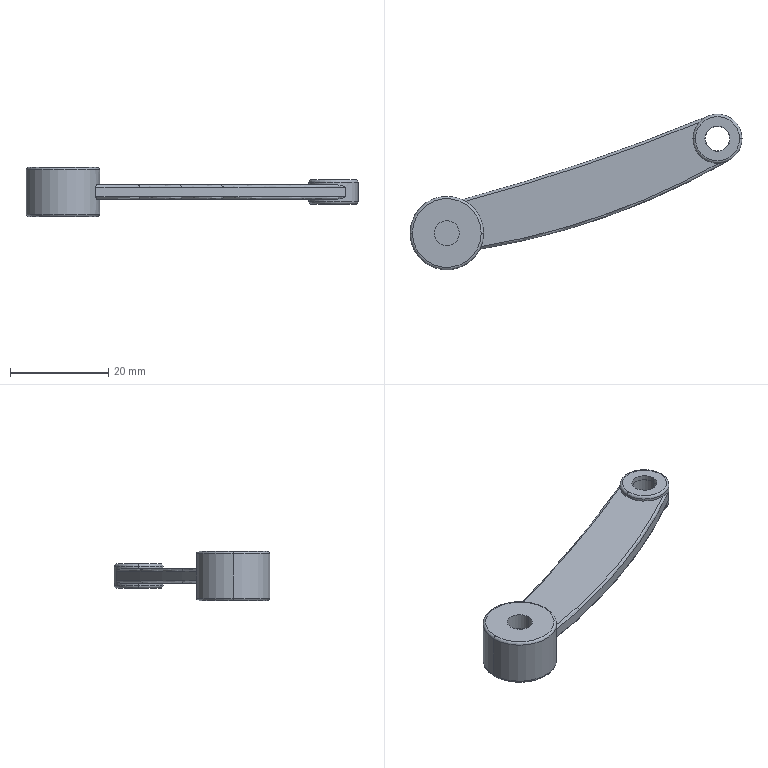Part | SolidWorks | features ICE 2, Extrusion 1, Fillet 1, MirrorPattern 1 | 1 solid | 38 faces | box 67.682 x 31.748 x 10 mm | volume 3550 mm3 | cylinder 16 | torus 12 | plane 10 | commonest cylinder face diameters 5.1 x8 5 x2 10 x2 15 x2 300 x1 800 x1
STEP:
#1=CARTESIAN_POINT('',(-7.5,0.,4.5));
#2=VERTEX_POINT('',#1);
#3=CARTESIAN_POINT('',(7.5,0.,4.5));
#4=VERTEX_POINT('',#3);
#5=CARTESIAN_POINT('',(0.,0.,4.5));
#6=DIRECTION('',(0.,0.,-1.));
#7=DIRECTION('',(1.,0.,0.));
#8=AXIS2_PLACEMENT_3D('',#5,#6,#7);
#9=CIRCLE('',#8,7.5);
#10=EDGE_CURVE('',#2,#4,#9,.T.);
#11=ORIENTED_EDGE('',*,*,#10,.F.);
#12=CARTESIAN_POINT('',(-7.,0.,5.));
#13=VERTEX_POINT('',#12);
#14=CARTESIAN_POINT('',(-7.,0.,4.5));
#15=DIRECTION('',(0.,1.,0.));
#16=DIRECTION('',(-1.,0.,0.));
#17=AXIS2_PLACEMENT_3D('',#14,#15,#16);
#18=CIRCLE('',#17,0.5);
#19=EDGE_CURVE('',#2,#13,#18,.T.);
#20=ORIENTED_EDGE('',*,*,#19,.T.);
#21=CARTESIAN_POINT('',(7.,0.,5.));
#22=VERTEX_POINT('',#21);
#23=CARTESIAN_POINT('',(0.,0.,5.));
#24=DIRECTION('',(0.,0.,1.));
#25=DIRECTION('',(1.,0.,0.));
#26=AXIS2_PLACEMENT_3D('',#23,#24,#25);
#27=CIRCLE('',#26,7.);
#28=EDGE_CURVE('',#22,#13,#27,.T.);
#29=ORIENTED_EDGE('',*,*,#28,.F.);
#30=CARTESIAN_POINT('',(7.,0.,4.5));
#31=DIRECTION('',(0.,-1.,0.));
#32=DIRECTION('',(0.,0.,-1.));
#33=AXIS2_PLACEMENT_3D('',#30,#31,#32);
#34=CIRCLE('',#33,0.5);
#35=EDGE_CURVE('',#4,#22,#34,.T.);
#36=ORIENTED_EDGE('',*,*,#35,.F.);
#37=EDGE_LOOP('',(#11,#20,#29,#36));
#38=FACE_OUTER_BOUND('',#37,.T.);
#39=CARTESIAN_POINT('',(0.,0.,4.5));
#40=DIRECTION('',(0.,0.,1.));
#41=DIRECTION('',(1.,0.,0.));
#42=AXIS2_PLACEMENT_3D('',#39,#40,#41);
#43=TOROIDAL_SURFACE('',#42,7.,0.5);
#44=ADVANCED_FACE('',(#38),#43,.T.);
#45=CARTESIAN_POINT('',(50.182,19.248,2.));
#46=VERTEX_POINT('',#45);
#47=CARTESIAN_POINT('',(60.182,19.248,2.));
#48=VERTEX_POINT('',#47);
#49=CARTESIAN_POINT('',(55.182,19.248,2.));
#50=DIRECTION('',(0.,0.,-1.));
#51=DIRECTION('',(1.,0.,0.));
#52=AXIS2_PLACEMENT_3D('',#49,#50,#51);
#53=CIRCLE('',#52,5.);
#54=EDGE_CURVE('',#46,#48,#53,.T.);
#55=ORIENTED_EDGE('',*,*,#54,.F.);
#56=CARTESIAN_POINT('',(50.682,19.248,2.5));
#57=VERTEX_POINT('',#56);
#58=CARTESIAN_POINT('',(50.682,19.248,2.));
#59=DIRECTION('',(0.,1.,0.));
#60=DIRECTION('',(-1.,0.,0.));
#61=AXIS2_PLACEMENT_3D('',#58,#59,#60);
#62=CIRCLE('',#61,0.5);
#63=EDGE_CURVE('',#46,#57,#62,.T.);
#64=ORIENTED_EDGE('',*,*,#63,.T.);
#65=CARTESIAN_POINT('',(59.682,19.248,2.5));
#66=VERTEX_POINT('',#65);
#67=CARTESIAN_POINT('',(55.182,19.248,2.5));
#68=DIRECTION('',(0.,0.,1.));
#69=DIRECTION('',(1.,0.,0.));
#70=AXIS2_PLACEMENT_3D('',#67,#68,#69);
#71=CIRCLE('',#70,4.5);
#72=EDGE_CURVE('',#66,#57,#71,.T.);
#73=ORIENTED_EDGE('',*,*,#72,.F.);
#74=CARTESIAN_POINT('',(59.682,19.248,2.));
#75=DIRECTION('',(0.,-1.,0.));
#76=DIRECTION('',(0.,0.,-1.));
#77=AXIS2_PLACEMENT_3D('',#74,#75,#76);
#78=CIRCLE('',#77,0.5);
#79=EDGE_CURVE('',#48,#66,#78,.T.);
#80=ORIENTED_EDGE('',*,*,#79,.F.);
#81=EDGE_LOOP('',(#55,#64,#73,#80));
#82=FACE_OUTER_BOUND('',#81,.T.);
#83=CARTESIAN_POINT('',(55.182,19.248,2.));
#84=DIRECTION('',(0.,0.,1.));
#85=DIRECTION('',(1.,0.,0.));
#86=AXIS2_PLACEMENT_3D('',#83,#84,#85);
#87=TOROIDAL_SURFACE('',#86,4.5,0.5);
#88=ADVANCED_FACE('',(#82),#87,.T.);
#89=CARTESIAN_POINT('',(60.182,19.248,-2.));
#90=VERTEX_POINT('',#89);
#91=CARTESIAN_POINT('',(50.182,19.248,-2.));
#92=VERTEX_POINT('',#91);
#93=CARTESIAN_POINT('',(55.182,19.248,-2.));
#94=DIRECTION('',(0.,0.,1.));
#95=DIRECTION('',(-1.,0.,0.));
#96=AXIS2_PLACEMENT_3D('',#93,#94,#95);
#97=CIRCLE('',#96,5.);
#98=EDGE_CURVE('',#90,#92,#97,.T.);
#99=ORIENTED_EDGE('',*,*,#98,.F.);
#100=CARTESIAN_POINT('',(59.682,19.248,-2.5));
#101=VERTEX_POINT('',#100);
#102=CARTESIAN_POINT('',(59.682,19.248,-2.));
#103=DIRECTION('',(0.,1.,0.));
#104=DIRECTION('',(-1.,0.,0.));
#105=AXIS2_PLACEMENT_3D('',#102,#103,#104);
#106=CIRCLE('',#105,0.5);
#107=EDGE_CURVE('',#90,#101,#106,.T.);
#108=ORIENTED_EDGE('',*,*,#107,.T.);
#109=CARTESIAN_POINT('',(50.682,19.248,-2.5));
#110=VERTEX_POINT('',#109);
#111=CARTESIAN_POINT('',(55.182,19.248,-2.5));
#112=DIRECTION('',(0.,0.,-1.));
#113=DIRECTION('',(-1.,0.,0.));
#114=AXIS2_PLACEMENT_3D('',#111,#112,#113);
#115=CIRCLE('',#114,4.5);
#116=EDGE_CURVE('',#110,#101,#115,.T.);
#117=ORIENTED_EDGE('',*,*,#116,.F.);
#118=CARTESIAN_POINT('',(50.682,19.248,-2.));
#119=DIRECTION('',(0.,-1.,0.));
#120=DIRECTION('',(0.,0.,-1.));
#121=AXIS2_PLACEMENT_3D('',#118,#119,#120);
#122=CIRCLE('',#121,0.5);
#123=EDGE_CURVE('',#92,#110,#122,.T.);
#124=ORIENTED_EDGE('',*,*,#123,.F.);
#125=EDGE_LOOP('',(#99,#108,#117,#124));
#126=FACE_OUTER_BOUND('',#125,.T.);
#127=CARTESIAN_POINT('',(55.182,19.248,-2.));
#128=DIRECTION('',(0.,0.,-1.));
#129=DIRECTION('',(-1.,0.,0.));
#130=AXIS2_PLACEMENT_3D('',#127,#128,#129);
#131=TOROIDAL_SURFACE('',#130,4.5,0.5);
#132=ADVANCED_FACE('',(#126),#131,.T.);
#133=CARTESIAN_POINT('',(-7.,0.,-5.));
#134=VERTEX_POINT('',#133);
#135=CARTESIAN_POINT('',(7.,0.,-5.));
#136=VERTEX_POINT('',#135);
#137=CARTESIAN_POINT('',(0.,0.,-5.));
#138=DIRECTION('',(0.,0.,-1.));
#139=DIRECTION('',(1.,0.,0.));
#140=AXIS2_PLACEMENT_3D('',#137,#138,#139);
#141=CIRCLE('',#140,7.);
#142=EDGE_CURVE('',#134,#136,#141,.T.);
#143=ORIENTED_EDGE('',*,*,#142,.F.);
#144=CARTESIAN_POINT('',(-7.5,0.,-4.5));
#145=VERTEX_POINT('',#144);
#146=CARTESIAN_POINT('',(-7.,0.,-4.5));
#147=DIRECTION('',(0.,1.,0.));
#148=DIRECTION('',(-1.,0.,0.));
#149=AXIS2_PLACEMENT_3D('',#146,#147,#148);
#150=CIRCLE('',#149,0.5);
#151=EDGE_CURVE('',#134,#145,#150,.T.);
#152=ORIENTED_EDGE('',*,*,#151,.T.);
#153=CARTESIAN_POINT('',(7.5,0.,-4.5));
#154=VERTEX_POINT('',#153);
#155=CARTESIAN_POINT('',(0.,0.,-4.5));
#156=DIRECTION('',(0.,0.,1.));
#157=DIRECTION('',(1.,0.,0.));
#158=AXIS2_PLACEMENT_3D('',#155,#156,#157);
#159=CIRCLE('',#158,7.5);
#160=EDGE_CURVE('',#154,#145,#159,.T.);
#161=ORIENTED_EDGE('',*,*,#160,.F.);
#162=CARTESIAN_POINT('',(7.,0.,-4.5));
#163=DIRECTION('',(0.,-1.,0.));
#164=DIRECTION('',(0.,0.,-1.));
#165=AXIS2_PLACEMENT_3D('',#162,#163,#164);
#166=CIRCLE('',#165,0.5);
#167=EDGE_CURVE('',#136,#154,#166,.T.);
#168=ORIENTED_EDGE('',*,*,#167,.F.);
#169=EDGE_LOOP('',(#143,#152,#161,#168));
#170=FACE_OUTER_BOUND('',#169,.T.);
#171=CARTESIAN_POINT('',(0.,0.,-4.5));
#172=DIRECTION('',(0.,0.,1.));
#173=DIRECTION('',(1.,0.,0.));
#174=AXIS2_PLACEMENT_3D('',#171,#172,#173);
#175=TOROIDAL_SURFACE('',#174,7.,0.5);
#176=ADVANCED_FACE('',(#170),#175,.T.);
#177=CARTESIAN_POINT('',(52.632,19.248,-2.5));
#178=VERTEX_POINT('',#177);
#179=CARTESIAN_POINT('',(57.732,19.248,-2.5));
#180=VERTEX_POINT('',#179);
#181=CARTESIAN_POINT('',(55.182,19.248,-2.5));
#182=DIRECTION('',(0.,0.,1.));
#183=DIRECTION('',(1.,0.,0.));
#184=AXIS2_PLACEMENT_3D('',#181,#182,#183);
#185=CIRCLE('',#184,2.55);
#186=EDGE_CURVE('',#178,#180,#185,.T.);
#187=ORIENTED_EDGE('',*,*,#186,.F.);
#188=CARTESIAN_POINT('',(52.632,19.248,-1.5));
#189=VERTEX_POINT('',#188);
#190=CARTESIAN_POINT('',(52.632,19.248,-2.5));
#191=DIRECTION('',(0.,0.,1.));
#192=VECTOR('',#191,1000.);
#193=LINE('',#190,#192);
#194=EDGE_CURVE('',#178,#189,#193,.T.);
#195=ORIENTED_EDGE('',*,*,#194,.T.);
#196=CARTESIAN_POINT('',(57.732,19.248,-1.5));
#197=VERTEX_POINT('',#196);
#198=CARTESIAN_POINT('',(55.182,19.248,-1.5));
#199=DIRECTION('',(0.,0.,1.));
#200=DIRECTION('',(1.,0.,0.));
#201=AXIS2_PLACEMENT_3D('',#198,#199,#200);
#202=CIRCLE('',#201,2.55);
#203=EDGE_CURVE('',#189,#197,#202,.T.);
#204=ORIENTED_EDGE('',*,*,#203,.T.);
#205=CARTESIAN_POINT('',(57.732,19.248,-2.5));
#206=DIRECTION('',(0.,0.,1.));
#207=VECTOR('',#206,1000.);
#208=LINE('',#205,#207);
#209=EDGE_CURVE('',#180,#197,#208,.T.);
#210=ORIENTED_EDGE('',*,*,#209,.F.);
#211=EDGE_LOOP('',(#187,#195,#204,#210));
#212=FACE_OUTER_BOUND('',#211,.T.);
#213=CARTESIAN_POINT('',(55.182,19.248,-2.5));
#214=DIRECTION('',(0.,0.,1.));
#215=DIRECTION('',(1.,0.,0.));
#216=AXIS2_PLACEMENT_3D('',#213,#214,#215);
#217=CYLINDRICAL_SURFACE('',#216,2.55);
#218=ADVANCED_FACE('',(#212),#217,.F.);
#219=CARTESIAN_POINT('',(52.632,19.248,2.5));
#220=VERTEX_POINT('',#219);
#221=CARTESIAN_POINT('',(57.732,19.248,2.5));
#222=VERTEX_POINT('',#221);
#223=CARTESIAN_POINT('',(55.182,19.248,2.5));
#224=DIRECTION('',(0.,0.,1.));
#225=DIRECTION('',(1.,0.,0.));
#226=AXIS2_PLACEMENT_3D('',#223,#224,#225);
#227=CIRCLE('',#226,2.55);
#228=EDGE_CURVE('',#220,#222,#227,.T.);
#229=ORIENTED_EDGE('',*,*,#228,.T.);
#230=CARTESIAN_POINT('',(57.732,19.248,1.5));
#231=VERTEX_POINT('',#230);
#232=CARTESIAN_POINT('',(57.732,19.248,2.5));
#233=DIRECTION('',(0.,0.,-1.));
#234=VECTOR('',#233,1000.);
#235=LINE('',#232,#234);
#236=EDGE_CURVE('',#222,#231,#235,.T.);
#237=ORIENTED_EDGE('',*,*,#236,.T.);
#238=CARTESIAN_POINT('',(52.632,19.248,1.5));
#239=VERTEX_POINT('',#238);
#240=CARTESIAN_POINT('',(55.182,19.248,1.5));
#241=DIRECTION('',(0.,0.,-1.));
#242=DIRECTION('',(1.,0.,0.));
#243=AXIS2_PLACEMENT_3D('',#240,#241,#242);
#244=CIRCLE('',#243,2.55);
#245=EDGE_CURVE('',#231,#239,#244,.T.);
#246=ORIENTED_EDGE('',*,*,#245,.T.);
#247=CARTESIAN_POINT('',(52.632,19.248,2.5));
#248=DIRECTION('',(0.,0.,-1.));
#249=VECTOR('',#248,1000.);
#250=LINE('',#247,#249);
#251=EDGE_CURVE('',#220,#239,#250,.T.);
#252=ORIENTED_EDGE('',*,*,#251,.F.);
#253=EDGE_LOOP('',(#229,#237,#246,#252));
#254=FACE_OUTER_BOUND('',#253,.T.);
#255=CARTESIAN_POINT('',(55.182,19.248,2.5));
#256=DIRECTION('',(0.,0.,-1.));
#257=DIRECTION('',(-1.,0.,0.));
#258=AXIS2_PLACEMENT_3D('',#255,#256,#257);
#259=CYLINDRICAL_SURFACE('',#258,2.55);
#260=ADVANCED_FACE('',(#254),#259,.F.);
#261=CARTESIAN_POINT('',(52.682,19.248,1.5));
#262=VERTEX_POINT('',#261);
#263=CARTESIAN_POINT('',(57.682,19.248,1.5));
#264=VERTEX_POINT('',#263);
#265=CARTESIAN_POINT('',(55.182,19.248,1.5));
#266=DIRECTION('',(0.,0.,1.));
#267=DIRECTION('',(1.,0.,0.));
#268=AXIS2_PLACEMENT_3D('',#265,#266,#267);
#269=CIRCLE('',#268,2.5);
#270=EDGE_CURVE('',#262,#264,#269,.T.);
#271=ORIENTED_EDGE('',*,*,#270,.T.);
#272=CARTESIAN_POINT('',(57.682,19.248,-1.5));
#273=VERTEX_POINT('',#272);
#274=CARTESIAN_POINT('',(57.682,19.248,1.5));
#275=DIRECTION('',(0.,0.,-1.));
#276=VECTOR('',#275,1000.);
#277=LINE('',#274,#276);
#278=EDGE_CURVE('',#264,#273,#277,.T.);
#279=ORIENTED_EDGE('',*,*,#278,.T.);
#280=CARTESIAN_POINT('',(52.682,19.248,-1.5));
#281=VERTEX_POINT('',#280);
#282=CARTESIAN_POINT('',(55.182,19.248,-1.5));
#283=DIRECTION('',(0.,0.,1.));
#284=DIRECTION('',(1.,0.,0.));
#285=AXIS2_PLACEMENT_3D('',#282,#283,#284);
#286=CIRCLE('',#285,2.5);
#287=EDGE_CURVE('',#281,#273,#286,.T.);
#288=ORIENTED_EDGE('',*,*,#287,.F.);
#289=CARTESIAN_POINT('',(52.682,19.248,1.5));
#290=DIRECTION('',(0.,0.,-1.));
#291=VECTOR('',#290,1000.);
#292=LINE('',#289,#291);
#293=EDGE_CURVE('',#262,#281,#292,.T.);
#294=ORIENTED_EDGE('',*,*,#293,.F.);
#295=EDGE_LOOP('',(#271,#279,#288,#294));
#296=FACE_OUTER_BOUND('',#295,.T.);
#297=CARTESIAN_POINT('',(55.182,19.248,1.5));
#298=DIRECTION('',(0.,0.,-1.));
#299=DIRECTION('',(-1.,0.,0.));
#300=AXIS2_PLACEMENT_3D('',#297,#298,#299);
#301=CYLINDRICAL_SURFACE('',#300,2.5);
#302=ADVANCED_FACE('',(#296),#301,.F.);
#303=ORIENTED_EDGE('',*,*,#54,.T.);
#304=CARTESIAN_POINT('',(60.182,19.248,1.5));
#305=DIRECTION('',(0.,0.,-1.));
#306=VECTOR('',#305,1000.);
#307=LINE('',#304,#306);
#308=EDGE_CURVE('',#48,#90,#307,.T.);
#309=ORIENTED_EDGE('',*,*,#308,.T.);
#310=ORIENTED_EDGE('',*,*,#98,.T.);
#311=CARTESIAN_POINT('',(50.182,19.248,-1.5));
#312=VERTEX_POINT('',#311);
#313=CARTESIAN_POINT('',(50.182,19.248,1.5));
#314=DIRECTION('',(0.,0.,-1.));
#315=VECTOR('',#314,1000.);
#316=LINE('',#313,#315);
#317=EDGE_CURVE('',#312,#92,#316,.T.);
#318=ORIENTED_EDGE('',*,*,#317,.F.);
#319=CARTESIAN_POINT('',(51.452,22.577,-1.5));
#320=VERTEX_POINT('',#319);
#321=CARTESIAN_POINT('',(55.182,19.248,-1.5));
#322=DIRECTION('',(0.,0.,1.));
#323=DIRECTION('',(1.,0.,0.));
#324=AXIS2_PLACEMENT_3D('',#321,#322,#323);
#325=CIRCLE('',#324,5.);
#326=EDGE_CURVE('',#320,#312,#325,.T.);
#327=ORIENTED_EDGE('',*,*,#326,.F.);
#328=CARTESIAN_POINT('',(53.263,23.865,-1.));
#329=VERTEX_POINT('',#328);
#330=CARTESIAN_POINT('',(51.452,22.577,-1.5));
#331=CARTESIAN_POINT('',(51.581,22.722,-1.5));
#332=CARTESIAN_POINT('',(51.716,22.857,-1.479));
#333=CARTESIAN_POINT('',(51.999,23.108,-1.418));
#334=CARTESIAN_POINT('',(52.147,23.226,-1.376));
#335=CARTESIAN_POINT('',(52.451,23.441,-1.281));
#336=CARTESIAN_POINT('',(52.608,23.538,-1.228));
#337=CARTESIAN_POINT('',(52.929,23.715,-1.117));
#338=CARTESIAN_POINT('',(53.095,23.795,-1.058));
#339=CARTESIAN_POINT('',(53.263,23.865,-1.));
#340=B_SPLINE_CURVE_WITH_KNOTS('',3,(#330,#331,#332,#333,#334,#335,#336,#337,#338,#339),.UNSPECIFIED.,.F.,.F.,(4,2,2,2,4),(0.,0.0005748,0.00115,0.001724,0.002299),.UNSPECIFIED.);
#341=EDGE_CURVE('',#320,#329,#340,.T.);
#342=ORIENTED_EDGE('',*,*,#341,.T.);
#343=CARTESIAN_POINT('',(53.263,23.865,1.));
#344=VERTEX_POINT('',#343);
#345=CARTESIAN_POINT('',(53.263,23.865,1.5));
#346=DIRECTION('',(0.,0.,-1.));
#347=VECTOR('',#346,1000.);
#348=LINE('',#345,#347);
#349=EDGE_CURVE('',#344,#329,#348,.T.);
#350=ORIENTED_EDGE('',*,*,#349,.F.);
#351=CARTESIAN_POINT('',(51.452,22.577,1.5));
#352=VERTEX_POINT('',#351);
#353=CARTESIAN_POINT('',(53.263,23.865,1.));
#354=CARTESIAN_POINT('',(53.095,23.795,1.058));
#355=CARTESIAN_POINT('',(52.929,23.715,1.117));
#356=CARTESIAN_POINT('',(52.608,23.538,1.228));
#357=CARTESIAN_POINT('',(52.451,23.441,1.281));
#358=CARTESIAN_POINT('',(52.147,23.226,1.376));
#359=CARTESIAN_POINT('',(51.999,23.108,1.418));
#360=CARTESIAN_POINT('',(51.716,22.857,1.479));
#361=CARTESIAN_POINT('',(51.581,22.722,1.5));
#362=CARTESIAN_POINT('',(51.452,22.577,1.5));
#363=B_SPLINE_CURVE_WITH_KNOTS('',3,(#353,#354,#355,#356,#357,#358,#359,#360,#361,#362),.UNSPECIFIED.,.F.,.F.,(4,2,2,2,4),(-0.00001405,0.0005603,0.001135,0.001709,0.002284),.UNSPECIFIED.);
#364=EDGE_CURVE('',#344,#352,#363,.T.);
#365=ORIENTED_EDGE('',*,*,#364,.T.);
#366=CARTESIAN_POINT('',(50.182,19.248,1.5));
#367=VERTEX_POINT('',#366);
#368=CARTESIAN_POINT('',(55.182,19.248,1.5));
#369=DIRECTION('',(0.,0.,1.));
#370=DIRECTION('',(1.,0.,0.));
#371=AXIS2_PLACEMENT_3D('',#368,#369,#370);
#372=CIRCLE('',#371,5.);
#373=EDGE_CURVE('',#352,#367,#372,.T.);
#374=ORIENTED_EDGE('',*,*,#373,.T.);
#375=CARTESIAN_POINT('',(50.182,19.248,1.5));
#376=DIRECTION('',(0.,0.,-1.));
#377=VECTOR('',#376,1000.);
#378=LINE('',#375,#377);
#379=EDGE_CURVE('',#46,#367,#378,.T.);
#380=ORIENTED_EDGE('',*,*,#379,.F.);
#381=EDGE_LOOP('',(#303,#309,#310,#318,#327,#342,#350,#365,#374,#380));
#382=FACE_OUTER_BOUND('',#381,.T.);
#383=CARTESIAN_POINT('',(55.182,19.248,1.5));
#384=DIRECTION('',(0.,0.,-1.));
#385=DIRECTION('',(-1.,0.,0.));
#386=AXIS2_PLACEMENT_3D('',#383,#384,#385);
#387=CYLINDRICAL_SURFACE('',#386,5.);
#388=ADVANCED_FACE('',(#382),#387,.T.);
#389=CARTESIAN_POINT('',(-2.55,0.,5.));
#390=VERTEX_POINT('',#389);
#391=CARTESIAN_POINT('',(2.55,0.,5.));
#392=VERTEX_POINT('',#391);
#393=CARTESIAN_POINT('',(0.,0.,5.));
#394=DIRECTION('',(0.,0.,1.));
#395=DIRECTION('',(1.,0.,0.));
#396=AXIS2_PLACEMENT_3D('',#393,#394,#395);
#397=CIRCLE('',#396,2.55);
#398=EDGE_CURVE('',#390,#392,#397,.T.);
#399=ORIENTED_EDGE('',*,*,#398,.T.);
#400=CARTESIAN_POINT('',(2.55,0.,1.5));
#401=VERTEX_POINT('',#400);
#402=CARTESIAN_POINT('',(2.55,0.,5.));
#403=DIRECTION('',(0.,0.,-1.));
#404=VECTOR('',#403,1000.);
#405=LINE('',#402,#404);
#406=EDGE_CURVE('',#392,#401,#405,.T.);
#407=ORIENTED_EDGE('',*,*,#406,.T.);
#408=CARTESIAN_POINT('',(-2.55,0.,1.5));
#409=VERTEX_POINT('',#408);
#410=CARTESIAN_POINT('',(0.,0.,1.5));
#411=DIRECTION('',(0.,0.,1.));
#412=DIRECTION('',(1.,0.,0.));
#413=AXIS2_PLACEMENT_3D('',#410,#411,#412);
#414=CIRCLE('',#413,2.55);
#415=EDGE_CURVE('',#409,#401,#414,.T.);
#416=ORIENTED_EDGE('',*,*,#415,.F.);
#417=CARTESIAN_POINT('',(-2.55,0.,5.));
#418=DIRECTION('',(0.,0.,-1.));
#419=VECTOR('',#418,1000.);
#420=LINE('',#417,#419);
#421=EDGE_CURVE('',#390,#409,#420,.T.);
#422=ORIENTED_EDGE('',*,*,#421,.F.);
#423=EDGE_LOOP('',(#399,#407,#416,#422));
#424=FACE_OUTER_BOUND('',#423,.T.);
#425=CARTESIAN_POINT('',(0.,0.,5.));
#426=DIRECTION('',(0.,0.,-1.));
#427=DIRECTION('',(-1.,0.,0.));
#428=AXIS2_PLACEMENT_3D('',#425,#426,#427);
#429=CYLINDRICAL_SURFACE('',#428,2.55);
#430=ADVANCED_FACE('',(#424),#429,.F.);
#431=ORIENTED_EDGE('',*,*,#10,.T.);
#432=CARTESIAN_POINT('',(7.5,0.,1.5));
#433=VERTEX_POINT('',#432);
#434=CARTESIAN_POINT('',(7.5,0.,5.));
#435=DIRECTION('',(0.,0.,-1.));
#436=VECTOR('',#435,1000.);
#437=LINE('',#434,#436);
#438=EDGE_CURVE('',#4,#433,#437,.T.);
#439=ORIENTED_EDGE('',*,*,#438,.T.);
#440=CARTESIAN_POINT('',(3.769,6.484,1.5));
#441=VERTEX_POINT('',#440);
#442=CARTESIAN_POINT('',(0.,0.,1.5));
#443=DIRECTION('',(0.,0.,1.));
#444=DIRECTION('',(1.,0.,0.));
#445=AXIS2_PLACEMENT_3D('',#442,#443,#444);
#446=CIRCLE('',#445,7.5);
#447=EDGE_CURVE('',#433,#441,#446,.T.);
#448=ORIENTED_EDGE('',*,*,#447,.T.);
#449=CARTESIAN_POINT('',(3.109,6.825,1.));
#450=VERTEX_POINT('',#449);
#451=CARTESIAN_POINT('',(3.769,6.484,1.5));
#452=CARTESIAN_POINT('',(3.698,6.526,1.5));
#453=CARTESIAN_POINT('',(3.627,6.565,1.49));
#454=CARTESIAN_POINT('',(3.488,6.64,1.451));
#455=CARTESIAN_POINT('',(3.419,6.676,1.422));
#456=CARTESIAN_POINT('',(3.292,6.739,1.342));
#457=CARTESIAN_POINT('',(3.232,6.768,1.291));
#458=CARTESIAN_POINT('',(3.14,6.811,1.162));
#459=CARTESIAN_POINT('',(3.109,6.825,1.083));
#460=CARTESIAN_POINT('',(3.109,6.825,1.));
#461=B_SPLINE_CURVE_WITH_KNOTS('',3,(#451,#452,#453,#454,#455,#456,#457,#458,#459,#460),.UNSPECIFIED.,.F.,.F.,(4,2,2,2,4),(0.,0.0002432,0.0004865,0.0007297,0.0009729),.UNSPECIFIED.);
#462=EDGE_CURVE('',#441,#450,#461,.T.);
#463=ORIENTED_EDGE('',*,*,#462,.T.);
#464=CARTESIAN_POINT('',(3.109,6.825,-1.));
#465=VERTEX_POINT('',#464);
#466=CARTESIAN_POINT('',(3.109,6.825,1.5));
#467=DIRECTION('',(0.,0.,-1.));
#468=VECTOR('',#467,1000.);
#469=LINE('',#466,#468);
#470=EDGE_CURVE('',#450,#465,#469,.T.);
#471=ORIENTED_EDGE('',*,*,#470,.T.);
#472=CARTESIAN_POINT('',(3.769,6.484,-1.5));
#473=VERTEX_POINT('',#472);
#474=CARTESIAN_POINT('',(3.109,6.825,-1.));
#475=CARTESIAN_POINT('',(3.109,6.825,-1.083));
#476=CARTESIAN_POINT('',(3.14,6.811,-1.161));
#477=CARTESIAN_POINT('',(3.232,6.768,-1.291));
#478=CARTESIAN_POINT('',(3.292,6.739,-1.342));
#479=CARTESIAN_POINT('',(3.483,6.644,-1.462));
#480=CARTESIAN_POINT('',(3.627,6.567,-1.5));
#481=CARTESIAN_POINT('',(3.769,6.484,-1.5));
#482=B_SPLINE_CURVE_WITH_KNOTS('',3,(#474,#475,#476,#477,#478,#479,#480,#481),.UNSPECIFIED.,.F.,.F.,(4,2,2,4),(0.,0.0002443,0.0004887,0.0009774),.UNSPECIFIED.);
#483=EDGE_CURVE('',#465,#473,#482,.T.);
#484=ORIENTED_EDGE('',*,*,#483,.T.);
#485=CARTESIAN_POINT('',(7.5,0.,-1.5));
#486=VERTEX_POINT('',#485);
#487=CARTESIAN_POINT('',(0.,0.,-1.5));
#488=DIRECTION('',(0.,0.,1.));
#489=DIRECTION('',(1.,0.,0.));
#490=AXIS2_PLACEMENT_3D('',#487,#488,#489);
#491=CIRCLE('',#490,7.5);
#492=EDGE_CURVE('',#486,#473,#491,.T.);
#493=ORIENTED_EDGE('',*,*,#492,.F.);
#494=CARTESIAN_POINT('',(7.5,0.,5.));
#495=DIRECTION('',(0.,0.,-1.));
#496=VECTOR('',#495,1000.);
#497=LINE('',#494,#496);
#498=EDGE_CURVE('',#486,#154,#497,.T.);
#499=ORIENTED_EDGE('',*,*,#498,.T.);
#500=ORIENTED_EDGE('',*,*,#160,.T.);
#501=CARTESIAN_POINT('',(-7.5,0.,5.));
#502=DIRECTION('',(0.,0.,-1.));
#503=VECTOR('',#502,1000.);
#504=LINE('',#501,#503);
#505=EDGE_CURVE('',#2,#145,#504,.T.);
#506=ORIENTED_EDGE('',*,*,#505,.F.);
#507=EDGE_LOOP('',(#431,#439,#448,#463,#471,#484,#493,#499,#500,#506));
#508=FACE_OUTER_BOUND('',#507,.T.);
#509=CARTESIAN_POINT('',(0.,0.,5.));
#510=DIRECTION('',(0.,0.,-1.));
#511=DIRECTION('',(-1.,0.,0.));
#512=AXIS2_PLACEMENT_3D('',#509,#510,#511);
#513=CYLINDRICAL_SURFACE('',#512,7.5);
#514=ADVANCED_FACE('',(#508),#513,.T.);
#515=CARTESIAN_POINT('',(-2.55,0.,-1.5));
#516=VERTEX_POINT('',#515);
#517=CARTESIAN_POINT('',(2.55,0.,-1.5));
#518=VERTEX_POINT('',#517);
#519=CARTESIAN_POINT('',(0.,0.,-1.5));
#520=DIRECTION('',(0.,0.,1.));
#521=DIRECTION('',(1.,0.,0.));
#522=AXIS2_PLACEMENT_3D('',#519,#520,#521);
#523=CIRCLE('',#522,2.55);
#524=EDGE_CURVE('',#516,#518,#523,.T.);
#525=ORIENTED_EDGE('',*,*,#524,.T.);
#526=CARTESIAN_POINT('',(2.55,0.,-5.));
#527=VERTEX_POINT('',#526);
#528=CARTESIAN_POINT('',(2.55,0.,5.));
#529=DIRECTION('',(0.,0.,-1.));
#530=VECTOR('',#529,1000.);
#531=LINE('',#528,#530);
#532=EDGE_CURVE('',#518,#527,#531,.T.);
#533=ORIENTED_EDGE('',*,*,#532,.T.);
#534=CARTESIAN_POINT('',(-2.55,0.,-5.));
#535=VERTEX_POINT('',#534);
#536=CARTESIAN_POINT('',(0.,0.,-5.));
#537=DIRECTION('',(0.,0.,1.));
#538=DIRECTION('',(1.,0.,0.));
#539=AXIS2_PLACEMENT_3D('',#536,#537,#538);
#540=CIRCLE('',#539,2.55);
#541=EDGE_CURVE('',#535,#527,#540,.T.);
#542=ORIENTED_EDGE('',*,*,#541,.F.);
#543=CARTESIAN_POINT('',(-2.55,0.,5.));
#544=DIRECTION('',(0.,0.,-1.));
#545=VECTOR('',#544,1000.);
#546=LINE('',#543,#545);
#547=EDGE_CURVE('',#516,#535,#546,.T.);
#548=ORIENTED_EDGE('',*,*,#547,.F.);
#549=EDGE_LOOP('',(#525,#533,#542,#548));
#550=FACE_OUTER_BOUND('',#549,.T.);
#551=CARTESIAN_POINT('',(0.,0.,5.));
#552=DIRECTION('',(0.,0.,-1.));
#553=DIRECTION('',(-1.,0.,0.));
#554=AXIS2_PLACEMENT_3D('',#551,#552,#553);
#555=CYLINDRICAL_SURFACE('',#554,2.55);
#556=ADVANCED_FACE('',(#550),#555,.F.);
#557=ORIENTED_EDGE('',*,*,#287,.T.);
#558=CARTESIAN_POINT('',(55.182,19.248,-1.5));
#559=DIRECTION('',(0.,0.,1.));
#560=DIRECTION('',(1.,0.,0.));
#561=AXIS2_PLACEMENT_3D('',#558,#559,#560);
#562=CIRCLE('',#561,2.5);
#563=EDGE_CURVE('',#273,#281,#562,.T.);
#564=ORIENTED_EDGE('',*,*,#563,.T.);
#565=EDGE_LOOP('',(#557,#564));
#566=FACE_BOUND('',#565,.T.);
#567=CARTESIAN_POINT('',(55.182,19.248,-1.5));
#568=DIRECTION('',(0.,0.,1.));
#569=DIRECTION('',(1.,0.,0.));
#570=AXIS2_PLACEMENT_3D('',#567,#568,#569);
#571=CIRCLE('',#570,2.55);
#572=EDGE_CURVE('',#197,#189,#571,.T.);
#573=ORIENTED_EDGE('',*,*,#572,.F.);
#574=ORIENTED_EDGE('',*,*,#203,.F.);
#575=EDGE_LOOP('',(#573,#574));
#576=FACE_OUTER_BOUND('',#575,.T.);
#577=CARTESIAN_POINT('',(-22.513,206.25,-1.5));
#578=DIRECTION('',(0.,0.,1.));
#579=DIRECTION('',(1.,0.,0.));
#580=AXIS2_PLACEMENT_3D('',#577,#578,#579);
#581=PLANE('',#580);
#582=ADVANCED_FACE('',(#566,#576),#581,.F.);
#583=ORIENTED_EDGE('',*,*,#270,.F.);
#584=CARTESIAN_POINT('',(55.182,19.248,1.5));
#585=DIRECTION('',(0.,0.,1.));
#586=DIRECTION('',(1.,0.,0.));
#587=AXIS2_PLACEMENT_3D('',#584,#585,#586);
#588=CIRCLE('',#587,2.5);
#589=EDGE_CURVE('',#264,#262,#588,.T.);
#590=ORIENTED_EDGE('',*,*,#589,.F.);
#591=EDGE_LOOP('',(#583,#590));
#592=FACE_BOUND('',#591,.T.);
#593=CARTESIAN_POINT('',(55.182,19.248,1.5));
#594=DIRECTION('',(0.,0.,-1.));
#595=DIRECTION('',(1.,0.,0.));
#596=AXIS2_PLACEMENT_3D('',#593,#594,#595);
#597=CIRCLE('',#596,2.55);
#598=EDGE_CURVE('',#239,#231,#597,.T.);
#599=ORIENTED_EDGE('',*,*,#598,.F.);
#600=ORIENTED_EDGE('',*,*,#245,.F.);
#601=EDGE_LOOP('',(#599,#600));
#602=FACE_OUTER_BOUND('',#601,.T.);
#603=CARTESIAN_POINT('',(-22.513,206.25,1.5));
#604=DIRECTION('',(0.,0.,1.));
#605=DIRECTION('',(1.,0.,0.));
#606=AXIS2_PLACEMENT_3D('',#603,#604,#605);
#607=PLANE('',#606);
#608=ADVANCED_FACE('',(#592,#602),#607,.T.);
#609=ORIENTED_EDGE('',*,*,#532,.F.);
#610=CARTESIAN_POINT('',(0.,0.,-1.5));
#611=DIRECTION('',(0.,0.,1.));
#612=DIRECTION('',(1.,0.,0.));
#613=AXIS2_PLACEMENT_3D('',#610,#611,#612);
#614=CIRCLE('',#613,2.55);
#615=EDGE_CURVE('',#518,#516,#614,.T.);
#616=ORIENTED_EDGE('',*,*,#615,.T.);
#617=ORIENTED_EDGE('',*,*,#547,.T.);
#618=CARTESIAN_POINT('',(0.,0.,-5.));
#619=DIRECTION('',(0.,0.,1.));
#620=DIRECTION('',(1.,0.,0.));
#621=AXIS2_PLACEMENT_3D('',#618,#619,#620);
#622=CIRCLE('',#621,2.55);
#623=EDGE_CURVE('',#527,#535,#622,.T.);
#624=ORIENTED_EDGE('',*,*,#623,.F.);
#625=EDGE_LOOP('',(#609,#616,#617,#624));
#626=FACE_OUTER_BOUND('',#625,.T.);
#627=CARTESIAN_POINT('',(0.,0.,5.));
#628=DIRECTION('',(0.,0.,-1.));
#629=DIRECTION('',(-1.,0.,0.));
#630=AXIS2_PLACEMENT_3D('',#627,#628,#629);
#631=CYLINDRICAL_SURFACE('',#630,2.55);
#632=ADVANCED_FACE('',(#626),#631,.F.);
#633=ORIENTED_EDGE('',*,*,#28,.T.);
#634=CARTESIAN_POINT('',(0.,0.,5.));
#635=DIRECTION('',(0.,0.,1.));
#636=DIRECTION('',(1.,0.,0.));
#637=AXIS2_PLACEMENT_3D('',#634,#635,#636);
#638=CIRCLE('',#637,7.);
#639=EDGE_CURVE('',#13,#22,#638,.T.);
#640=ORIENTED_EDGE('',*,*,#639,.T.);
#641=EDGE_LOOP('',(#633,#640));
#642=FACE_OUTER_BOUND('',#641,.T.);
#643=ORIENTED_EDGE('',*,*,#398,.F.);
#644=CARTESIAN_POINT('',(0.,0.,5.));
#645=DIRECTION('',(0.,0.,1.));
#646=DIRECTION('',(1.,0.,0.));
#647=AXIS2_PLACEMENT_3D('',#644,#645,#646);
#648=CIRCLE('',#647,2.55);
#649=EDGE_CURVE('',#392,#390,#648,.T.);
#650=ORIENTED_EDGE('',*,*,#649,.F.);
#651=EDGE_LOOP('',(#643,#650));
#652=FACE_BOUND('',#651,.T.);
#653=CARTESIAN_POINT('',(0.,0.,5.));
#654=DIRECTION('',(0.,0.,1.));
#655=DIRECTION('',(1.,0.,0.));
#656=AXIS2_PLACEMENT_3D('',#653,#654,#655);
#657=PLANE('',#656);
#658=ADVANCED_FACE('',(#642,#652),#657,.T.);
#659=CARTESIAN_POINT('',(0.,0.,-5.));
#660=DIRECTION('',(0.,0.,-1.));
#661=DIRECTION('',(1.,0.,0.));
#662=AXIS2_PLACEMENT_3D('',#659,#660,#661);
#663=CIRCLE('',#662,7.);
#664=EDGE_CURVE('',#136,#134,#663,.T.);
#665=ORIENTED_EDGE('',*,*,#664,.T.);
#666=ORIENTED_EDGE('',*,*,#142,.T.);
#667=EDGE_LOOP('',(#665,#666));
#668=FACE_OUTER_BOUND('',#667,.T.);
#669=ORIENTED_EDGE('',*,*,#541,.T.);
#670=ORIENTED_EDGE('',*,*,#623,.T.);
#671=EDGE_LOOP('',(#669,#670));
#672=FACE_BOUND('',#671,.T.);
#673=CARTESIAN_POINT('',(0.,0.,-5.));
#674=DIRECTION('',(0.,0.,1.));
#675=DIRECTION('',(1.,0.,0.));
#676=AXIS2_PLACEMENT_3D('',#673,#674,#675);
#677=PLANE('',#676);
#678=ADVANCED_FACE('',(#668,#672),#677,.F.);
#679=ORIENTED_EDGE('',*,*,#438,.F.);
#680=CARTESIAN_POINT('',(0.,0.,4.5));
#681=DIRECTION('',(0.,0.,-1.));
#682=DIRECTION('',(1.,0.,0.));
#683=AXIS2_PLACEMENT_3D('',#680,#681,#682);
#684=CIRCLE('',#683,7.5);
#685=EDGE_CURVE('',#4,#2,#684,.T.);
#686=ORIENTED_EDGE('',*,*,#685,.T.);
#687=ORIENTED_EDGE('',*,*,#505,.T.);
#688=CARTESIAN_POINT('',(0.,0.,-4.5));
#689=DIRECTION('',(0.,0.,1.));
#690=DIRECTION('',(1.,0.,0.));
#691=AXIS2_PLACEMENT_3D('',#688,#689,#690);
#692=CIRCLE('',#691,7.5);
#693=EDGE_CURVE('',#145,#154,#692,.T.);
#694=ORIENTED_EDGE('',*,*,#693,.T.);
#695=ORIENTED_EDGE('',*,*,#498,.F.);
#696=CARTESIAN_POINT('',(6.985,-2.732,-1.5));
#697=VERTEX_POINT('',#696);
#698=CARTESIAN_POINT('',(0.,0.,-1.5));
#699=DIRECTION('',(0.,0.,1.));
#700=DIRECTION('',(1.,0.,0.));
#701=AXIS2_PLACEMENT_3D('',#698,#699,#700);
#702=CIRCLE('',#701,7.5);
#703=EDGE_CURVE('',#697,#486,#702,.T.);
#704=ORIENTED_EDGE('',*,*,#703,.F.);
#705=CARTESIAN_POINT('',(6.745,-3.278,-1.));
#706=VERTEX_POINT('',#705);
#707=CARTESIAN_POINT('',(6.985,-2.732,-1.5));
#708=CARTESIAN_POINT('',(6.958,-2.8,-1.5));
#709=CARTESIAN_POINT('',(6.932,-2.865,-1.489));
#710=CARTESIAN_POINT('',(6.878,-2.99,-1.444));
#711=CARTESIAN_POINT('',(6.852,-3.05,-1.411));
#712=CARTESIAN_POINT('',(6.805,-3.153,-1.324));
#713=CARTESIAN_POINT('',(6.784,-3.198,-1.27));
#714=CARTESIAN_POINT('',(6.754,-3.261,-1.143));
#715=CARTESIAN_POINT('',(6.745,-3.278,-1.073));
#716=CARTESIAN_POINT('',(6.745,-3.278,-1.));
#717=B_SPLINE_CURVE_WITH_KNOTS('',3,(#707,#708,#709,#710,#711,#712,#713,#714,#715,#716),.UNSPECIFIED.,.F.,.F.,(4,2,2,2,4),(0.,0.0002133,0.0004266,0.0006399,0.0008533),.UNSPECIFIED.);
#718=EDGE_CURVE('',#697,#706,#717,.T.);
#719=ORIENTED_EDGE('',*,*,#718,.T.);
#720=CARTESIAN_POINT('',(6.745,-3.278,1.));
#721=VERTEX_POINT('',#720);
#722=CARTESIAN_POINT('',(6.745,-3.278,1.5));
#723=DIRECTION('',(0.,0.,-1.));
#724=VECTOR('',#723,1000.);
#725=LINE('',#722,#724);
#726=EDGE_CURVE('',#721,#706,#725,.T.);
#727=ORIENTED_EDGE('',*,*,#726,.F.);
#728=CARTESIAN_POINT('',(6.985,-2.732,1.5));
#729=VERTEX_POINT('',#728);
#730=CARTESIAN_POINT('',(6.745,-3.278,1.));
#731=CARTESIAN_POINT('',(6.745,-3.278,1.073));
#732=CARTESIAN_POINT('',(6.754,-3.261,1.143));
#733=CARTESIAN_POINT('',(6.784,-3.198,1.269));
#734=CARTESIAN_POINT('',(6.805,-3.154,1.323));
#735=CARTESIAN_POINT('',(6.876,-2.998,1.455));
#736=CARTESIAN_POINT('',(6.932,-2.867,1.5));
#737=CARTESIAN_POINT('',(6.985,-2.732,1.5));
#738=B_SPLINE_CURVE_WITH_KNOTS('',3,(#730,#731,#732,#733,#734,#735,#736,#737),.UNSPECIFIED.,.F.,.F.,(4,2,2,4),(0.,0.0002142,0.0004283,0.0008566),.UNSPECIFIED.);
#739=EDGE_CURVE('',#721,#729,#738,.T.);
#740=ORIENTED_EDGE('',*,*,#739,.T.);
#741=CARTESIAN_POINT('',(0.,0.,1.5));
#742=DIRECTION('',(0.,0.,1.));
#743=DIRECTION('',(1.,0.,0.));
#744=AXIS2_PLACEMENT_3D('',#741,#742,#743);
#745=CIRCLE('',#744,7.5);
#746=EDGE_CURVE('',#729,#433,#745,.T.);
#747=ORIENTED_EDGE('',*,*,#746,.T.);
#748=EDGE_LOOP('',(#679,#686,#687,#694,#695,#704,#719,#727,#740,#747));
#749=FACE_OUTER_BOUND('',#748,.T.);
#750=CARTESIAN_POINT('',(0.,0.,5.));
#751=DIRECTION('',(0.,0.,-1.));
#752=DIRECTION('',(-1.,0.,0.));
#753=AXIS2_PLACEMENT_3D('',#750,#751,#752);
#754=CYLINDRICAL_SURFACE('',#753,7.5);
#755=ADVANCED_FACE('',(#749),#754,.T.);
#756=ORIENTED_EDGE('',*,*,#406,.F.);
#757=ORIENTED_EDGE('',*,*,#649,.T.);
#758=ORIENTED_EDGE('',*,*,#421,.T.);
#759=CARTESIAN_POINT('',(0.,0.,1.5));
#760=DIRECTION('',(0.,0.,1.));
#761=DIRECTION('',(1.,0.,0.));
#762=AXIS2_PLACEMENT_3D('',#759,#760,#761);
#763=CIRCLE('',#762,2.55);
#764=EDGE_CURVE('',#401,#409,#763,.T.);
#765=ORIENTED_EDGE('',*,*,#764,.F.);
#766=EDGE_LOOP('',(#756,#757,#758,#765));
#767=FACE_OUTER_BOUND('',#766,.T.);
#768=CARTESIAN_POINT('',(0.,0.,5.));
#769=DIRECTION('',(0.,0.,-1.));
#770=DIRECTION('',(-1.,0.,0.));
#771=AXIS2_PLACEMENT_3D('',#768,#769,#770);
#772=CYLINDRICAL_SURFACE('',#771,2.55);
#773=ADVANCED_FACE('',(#767),#772,.F.);
#774=ORIENTED_EDGE('',*,*,#524,.F.);
#775=ORIENTED_EDGE('',*,*,#615,.F.);
#776=EDGE_LOOP('',(#774,#775));
#777=FACE_OUTER_BOUND('',#776,.T.);
#778=CARTESIAN_POINT('',(-22.513,206.25,-1.5));
#779=DIRECTION('',(0.,0.,1.));
#780=DIRECTION('',(1.,0.,0.));
#781=AXIS2_PLACEMENT_3D('',#778,#779,#780);
#782=PLANE('',#781);
#783=ADVANCED_FACE('',(#777),#782,.F.);
#784=ORIENTED_EDGE('',*,*,#415,.T.);
#785=ORIENTED_EDGE('',*,*,#764,.T.);
#786=EDGE_LOOP('',(#784,#785));
#787=FACE_OUTER_BOUND('',#786,.T.);
#788=CARTESIAN_POINT('',(-22.513,206.25,1.5));
#789=DIRECTION('',(0.,0.,1.));
#790=DIRECTION('',(1.,0.,0.));
#791=AXIS2_PLACEMENT_3D('',#788,#789,#790);
#792=PLANE('',#791);
#793=ADVANCED_FACE('',(#787),#792,.T.);
#794=ORIENTED_EDGE('',*,*,#746,.F.);
#795=CARTESIAN_POINT('',(55.511,14.259,1.5));
#796=VERTEX_POINT('',#795);
#797=CARTESIAN_POINT('',(-17.421,144.762,1.5));
#798=DIRECTION('',(0.,0.,1.));
#799=DIRECTION('',(1.,0.,0.));
#800=AXIS2_PLACEMENT_3D('',#797,#798,#799);
#801=CIRCLE('',#800,149.5);
#802=EDGE_CURVE('',#729,#796,#801,.T.);
#803=ORIENTED_EDGE('',*,*,#802,.T.);
#804=CARTESIAN_POINT('',(55.182,19.248,1.5));
#805=DIRECTION('',(0.,0.,1.));
#806=DIRECTION('',(1.,0.,0.));
#807=AXIS2_PLACEMENT_3D('',#804,#805,#806);
#808=CIRCLE('',#807,5.);
#809=EDGE_CURVE('',#367,#796,#808,.T.);
#810=ORIENTED_EDGE('',*,*,#809,.F.);
#811=ORIENTED_EDGE('',*,*,#373,.F.);
#812=CARTESIAN_POINT('',(-100.208,393.252,1.5));
#813=DIRECTION('',(0.,0.,-1.));
#814=DIRECTION('',(1.,0.,0.));
#815=AXIS2_PLACEMENT_3D('',#812,#813,#814);
#816=CIRCLE('',#815,400.5);
#817=EDGE_CURVE('',#352,#441,#816,.T.);
#818=ORIENTED_EDGE('',*,*,#817,.T.);
#819=ORIENTED_EDGE('',*,*,#447,.F.);
#820=EDGE_LOOP('',(#794,#803,#810,#811,#818,#819));
#821=FACE_OUTER_BOUND('',#820,.T.);
#822=CARTESIAN_POINT('',(-22.513,206.25,1.5));
#823=DIRECTION('',(0.,0.,1.));
#824=DIRECTION('',(1.,0.,0.));
#825=AXIS2_PLACEMENT_3D('',#822,#823,#824);
#826=PLANE('',#825);
#827=ADVANCED_FACE('',(#821),#826,.T.);
#828=ORIENTED_EDGE('',*,*,#326,.T.);
#829=CARTESIAN_POINT('',(55.511,14.259,-1.5));
#830=VERTEX_POINT('',#829);
#831=CARTESIAN_POINT('',(55.182,19.248,-1.5));
#832=DIRECTION('',(0.,0.,1.));
#833=DIRECTION('',(1.,0.,0.));
#834=AXIS2_PLACEMENT_3D('',#831,#832,#833);
#835=CIRCLE('',#834,5.);
#836=EDGE_CURVE('',#312,#830,#835,.T.);
#837=ORIENTED_EDGE('',*,*,#836,.T.);
#838=CARTESIAN_POINT('',(-17.421,144.762,-1.5));
#839=DIRECTION('',(0.,0.,-1.));
#840=DIRECTION('',(1.,0.,0.));
#841=AXIS2_PLACEMENT_3D('',#838,#839,#840);
#842=CIRCLE('',#841,149.5);
#843=EDGE_CURVE('',#830,#697,#842,.T.);
#844=ORIENTED_EDGE('',*,*,#843,.T.);
#845=ORIENTED_EDGE('',*,*,#703,.T.);
#846=ORIENTED_EDGE('',*,*,#492,.T.);
#847=CARTESIAN_POINT('',(-100.208,393.252,-1.5));
#848=DIRECTION('',(0.,0.,1.));
#849=DIRECTION('',(1.,0.,0.));
#850=AXIS2_PLACEMENT_3D('',#847,#848,#849);
#851=CIRCLE('',#850,400.5);
#852=EDGE_CURVE('',#473,#320,#851,.T.);
#853=ORIENTED_EDGE('',*,*,#852,.T.);
#854=EDGE_LOOP('',(#828,#837,#844,#845,#846,#853));
#855=FACE_OUTER_BOUND('',#854,.T.);
#856=CARTESIAN_POINT('',(-22.513,206.25,-1.5));
#857=DIRECTION('',(0.,0.,1.));
#858=DIRECTION('',(1.,0.,0.));
#859=AXIS2_PLACEMENT_3D('',#856,#857,#858);
#860=PLANE('',#859);
#861=ADVANCED_FACE('',(#855),#860,.F.);
#862=ORIENTED_EDGE('',*,*,#349,.T.);
#863=CARTESIAN_POINT('',(-100.208,393.252,-1.));
#864=DIRECTION('',(0.,0.,-1.));
#865=DIRECTION('',(1.,0.,0.));
#866=AXIS2_PLACEMENT_3D('',#863,#864,#865);
#867=CIRCLE('',#866,400.);
#868=EDGE_CURVE('',#329,#465,#867,.T.);
#869=ORIENTED_EDGE('',*,*,#868,.T.);
#870=ORIENTED_EDGE('',*,*,#470,.F.);
#871=CARTESIAN_POINT('',(-100.208,393.252,1.));
#872=DIRECTION('',(0.,0.,1.));
#873=DIRECTION('',(1.,0.,0.));
#874=AXIS2_PLACEMENT_3D('',#871,#872,#873);
#875=CIRCLE('',#874,400.);
#876=EDGE_CURVE('',#450,#344,#875,.T.);
#877=ORIENTED_EDGE('',*,*,#876,.T.);
#878=EDGE_LOOP('',(#862,#869,#870,#877));
#879=FACE_OUTER_BOUND('',#878,.T.);
#880=CARTESIAN_POINT('',(-100.208,393.252,1.5));
#881=DIRECTION('',(0.,0.,-1.));
#882=DIRECTION('',(-1.,0.,0.));
#883=AXIS2_PLACEMENT_3D('',#880,#881,#882);
#884=CYLINDRICAL_SURFACE('',#883,400.);
#885=ADVANCED_FACE('',(#879),#884,.F.);
#886=ORIENTED_EDGE('',*,*,#726,.T.);
#887=CARTESIAN_POINT('',(57.685,14.92,-1.));
#888=VERTEX_POINT('',#887);
#889=CARTESIAN_POINT('',(-17.421,144.762,-1.));
#890=DIRECTION('',(0.,0.,1.));
#891=DIRECTION('',(1.,0.,0.));
#892=AXIS2_PLACEMENT_3D('',#889,#890,#891);
#893=CIRCLE('',#892,150.);
#894=EDGE_CURVE('',#706,#888,#893,.T.);
#895=ORIENTED_EDGE('',*,*,#894,.T.);
#896=CARTESIAN_POINT('',(57.685,14.92,1.));
#897=VERTEX_POINT('',#896);
#898=CARTESIAN_POINT('',(57.685,14.92,1.5));
#899=DIRECTION('',(0.,0.,-1.));
#900=VECTOR('',#899,1000.);
#901=LINE('',#898,#900);
#902=EDGE_CURVE('',#897,#888,#901,.T.);
#903=ORIENTED_EDGE('',*,*,#902,.F.);
#904=CARTESIAN_POINT('',(-17.421,144.762,1.));
#905=DIRECTION('',(0.,0.,-1.));
#906=DIRECTION('',(1.,0.,0.));
#907=AXIS2_PLACEMENT_3D('',#904,#905,#906);
#908=CIRCLE('',#907,150.);
#909=EDGE_CURVE('',#897,#721,#908,.T.);
#910=ORIENTED_EDGE('',*,*,#909,.T.);
#911=EDGE_LOOP('',(#886,#895,#903,#910));
#912=FACE_OUTER_BOUND('',#911,.T.);
#913=CARTESIAN_POINT('',(-17.421,144.762,1.5));
#914=DIRECTION('',(0.,0.,-1.));
#915=DIRECTION('',(-1.,0.,0.));
#916=AXIS2_PLACEMENT_3D('',#913,#914,#915);
#917=CYLINDRICAL_SURFACE('',#916,150.);
#918=ADVANCED_FACE('',(#912),#917,.T.);
#919=ORIENTED_EDGE('',*,*,#308,.F.);
#920=CARTESIAN_POINT('',(55.182,19.248,2.));
#921=DIRECTION('',(0.,0.,-1.));
#922=DIRECTION('',(1.,0.,0.));
#923=AXIS2_PLACEMENT_3D('',#920,#921,#922);
#924=CIRCLE('',#923,5.);
#925=EDGE_CURVE('',#48,#46,#924,.T.);
#926=ORIENTED_EDGE('',*,*,#925,.T.);
#927=ORIENTED_EDGE('',*,*,#379,.T.);
#928=ORIENTED_EDGE('',*,*,#809,.T.);
#929=CARTESIAN_POINT('',(55.511,14.259,1.5));
#930=CARTESIAN_POINT('',(55.709,14.272,1.5));
#931=CARTESIAN_POINT('',(55.902,14.296,1.479));
#932=CARTESIAN_POINT('',(56.283,14.367,1.418));
#933=CARTESIAN_POINT('',(56.471,14.413,1.376));
#934=CARTESIAN_POINT('',(56.835,14.525,1.281));
#935=CARTESIAN_POINT('',(57.011,14.591,1.228));
#936=CARTESIAN_POINT('',(57.355,14.741,1.117));
#937=CARTESIAN_POINT('',(57.524,14.826,1.058));
#938=CARTESIAN_POINT('',(57.685,14.92,1.));
#939=B_SPLINE_CURVE_WITH_KNOTS('',3,(#929,#930,#931,#932,#933,#934,#935,#936,#937,#938),.UNSPECIFIED.,.F.,.F.,(4,2,2,2,4),(0.,0.0005871,0.001174,0.001761,0.002349),.UNSPECIFIED.);
#940=EDGE_CURVE('',#796,#897,#939,.T.);
#941=ORIENTED_EDGE('',*,*,#940,.T.);
#942=ORIENTED_EDGE('',*,*,#902,.T.);
#943=CARTESIAN_POINT('',(57.685,14.92,-1.));
#944=CARTESIAN_POINT('',(57.524,14.826,-1.058));
#945=CARTESIAN_POINT('',(57.355,14.741,-1.117));
#946=CARTESIAN_POINT('',(57.011,14.591,-1.228));
#947=CARTESIAN_POINT('',(56.835,14.525,-1.281));
#948=CARTESIAN_POINT('',(56.471,14.413,-1.376));
#949=CARTESIAN_POINT('',(56.283,14.367,-1.418));
#950=CARTESIAN_POINT('',(55.902,14.296,-1.479));
#951=CARTESIAN_POINT('',(55.709,14.272,-1.5));
#952=CARTESIAN_POINT('',(55.511,14.259,-1.5));
#953=B_SPLINE_CURVE_WITH_KNOTS('',3,(#943,#944,#945,#946,#947,#948,#949,#950,#951,#952),.UNSPECIFIED.,.F.,.F.,(4,2,2,2,4),(-0.00001438,0.0005722,0.001159,0.001745,0.002332),.UNSPECIFIED.);
#954=EDGE_CURVE('',#888,#830,#953,.T.);
#955=ORIENTED_EDGE('',*,*,#954,.T.);
#956=ORIENTED_EDGE('',*,*,#836,.F.);
#957=ORIENTED_EDGE('',*,*,#317,.T.);
#958=CARTESIAN_POINT('',(55.182,19.248,-2.));
#959=DIRECTION('',(0.,0.,1.));
#960=DIRECTION('',(-1.,0.,0.));
#961=AXIS2_PLACEMENT_3D('',#958,#959,#960);
#962=CIRCLE('',#961,5.);
#963=EDGE_CURVE('',#92,#90,#962,.T.);
#964=ORIENTED_EDGE('',*,*,#963,.T.);
#965=EDGE_LOOP('',(#919,#926,#927,#928,#941,#942,#955,#956,#957,#964));
#966=FACE_OUTER_BOUND('',#965,.T.);
#967=CARTESIAN_POINT('',(55.182,19.248,1.5));
#968=DIRECTION('',(0.,0.,-1.));
#969=DIRECTION('',(-1.,0.,0.));
#970=AXIS2_PLACEMENT_3D('',#967,#968,#969);
#971=CYLINDRICAL_SURFACE('',#970,5.);
#972=ADVANCED_FACE('',(#966),#971,.T.);
#973=ORIENTED_EDGE('',*,*,#278,.F.);
#974=ORIENTED_EDGE('',*,*,#589,.T.);
#975=ORIENTED_EDGE('',*,*,#293,.T.);
#976=ORIENTED_EDGE('',*,*,#563,.F.);
#977=EDGE_LOOP('',(#973,#974,#975,#976));
#978=FACE_OUTER_BOUND('',#977,.T.);
#979=CARTESIAN_POINT('',(55.182,19.248,1.5));
#980=DIRECTION('',(0.,0.,-1.));
#981=DIRECTION('',(-1.,0.,0.));
#982=AXIS2_PLACEMENT_3D('',#979,#980,#981);
#983=CYLINDRICAL_SURFACE('',#982,2.5);
#984=ADVANCED_FACE('',(#978),#983,.F.);
#985=ORIENTED_EDGE('',*,*,#72,.T.);
#986=CARTESIAN_POINT('',(55.182,19.248,2.5));
#987=DIRECTION('',(0.,0.,1.));
#988=DIRECTION('',(1.,0.,0.));
#989=AXIS2_PLACEMENT_3D('',#986,#987,#988);
#990=CIRCLE('',#989,4.5);
#991=EDGE_CURVE('',#57,#66,#990,.T.);
#992=ORIENTED_EDGE('',*,*,#991,.T.);
#993=EDGE_LOOP('',(#985,#992));
#994=FACE_OUTER_BOUND('',#993,.T.);
#995=ORIENTED_EDGE('',*,*,#228,.F.);
#996=CARTESIAN_POINT('',(55.182,19.248,2.5));
#997=DIRECTION('',(0.,0.,1.));
#998=DIRECTION('',(1.,0.,0.));
#999=AXIS2_PLACEMENT_3D('',#996,#997,#998);
#1000=CIRCLE('',#999,2.55);
#1001=EDGE_CURVE('',#222,#220,#1000,.T.);
#1002=ORIENTED_EDGE('',*,*,#1001,.F.);
#1003=EDGE_LOOP('',(#995,#1002));
#1004=FACE_BOUND('',#1003,.T.);
#1005=CARTESIAN_POINT('',(55.182,19.248,2.5));
#1006=DIRECTION('',(0.,0.,1.));
#1007=DIRECTION('',(1.,0.,0.));
#1008=AXIS2_PLACEMENT_3D('',#1005,#1006,#1007);
#1009=PLANE('',#1008);
#1010=ADVANCED_FACE('',(#994,#1004),#1009,.T.);
#1011=ORIENTED_EDGE('',*,*,#236,.F.);
#1012=ORIENTED_EDGE('',*,*,#1001,.T.);
#1013=ORIENTED_EDGE('',*,*,#251,.T.);
#1014=ORIENTED_EDGE('',*,*,#598,.T.);
#1015=EDGE_LOOP('',(#1011,#1012,#1013,#1014));
#1016=FACE_OUTER_BOUND('',#1015,.T.);
#1017=CARTESIAN_POINT('',(55.182,19.248,2.5));
#1018=DIRECTION('',(0.,0.,-1.));
#1019=DIRECTION('',(-1.,0.,0.));
#1020=AXIS2_PLACEMENT_3D('',#1017,#1018,#1019);
#1021=CYLINDRICAL_SURFACE('',#1020,2.55);
#1022=ADVANCED_FACE('',(#1016),#1021,.F.);
#1023=ORIENTED_EDGE('',*,*,#116,.T.);
#1024=CARTESIAN_POINT('',(55.182,19.248,-2.5));
#1025=DIRECTION('',(0.,0.,-1.));
#1026=DIRECTION('',(-1.,0.,0.));
#1027=AXIS2_PLACEMENT_3D('',#1024,#1025,#1026);
#1028=CIRCLE('',#1027,4.5);
#1029=EDGE_CURVE('',#101,#110,#1028,.T.);
#1030=ORIENTED_EDGE('',*,*,#1029,.T.);
#1031=EDGE_LOOP('',(#1023,#1030));
#1032=FACE_OUTER_BOUND('',#1031,.T.);
#1033=CARTESIAN_POINT('',(55.182,19.248,-2.5));
#1034=DIRECTION('',(0.,0.,1.));
#1035=DIRECTION('',(1.,0.,0.));
#1036=AXIS2_PLACEMENT_3D('',#1033,#1034,#1035);
#1037=CIRCLE('',#1036,2.55);
#1038=EDGE_CURVE('',#180,#178,#1037,.T.);
#1039=ORIENTED_EDGE('',*,*,#1038,.T.);
#1040=ORIENTED_EDGE('',*,*,#186,.T.);
#1041=EDGE_LOOP('',(#1039,#1040));
#1042=FACE_BOUND('',#1041,.T.);
#1043=CARTESIAN_POINT('',(55.182,19.248,-2.5));
#1044=DIRECTION('',(0.,0.,-1.));
#1045=DIRECTION('',(1.,0.,0.));
#1046=AXIS2_PLACEMENT_3D('',#1043,#1044,#1045);
#1047=PLANE('',#1046);
#1048=ADVANCED_FACE('',(#1032,#1042),#1047,.T.);
#1049=ORIENTED_EDGE('',*,*,#194,.F.);
#1050=ORIENTED_EDGE('',*,*,#1038,.F.);
#1051=ORIENTED_EDGE('',*,*,#209,.T.);
#1052=ORIENTED_EDGE('',*,*,#572,.T.);
#1053=EDGE_LOOP('',(#1049,#1050,#1051,#1052));
#1054=FACE_OUTER_BOUND('',#1053,.T.);
#1055=CARTESIAN_POINT('',(55.182,19.248,-2.5));
#1056=DIRECTION('',(0.,0.,1.));
#1057=DIRECTION('',(1.,0.,0.));
#1058=AXIS2_PLACEMENT_3D('',#1055,#1056,#1057);
#1059=CYLINDRICAL_SURFACE('',#1058,2.55);
#1060=ADVANCED_FACE('',(#1054),#1059,.F.);
#1061=ORIENTED_EDGE('',*,*,#151,.F.);
#1062=ORIENTED_EDGE('',*,*,#664,.F.);
#1063=ORIENTED_EDGE('',*,*,#167,.T.);
#1064=ORIENTED_EDGE('',*,*,#693,.F.);
#1065=EDGE_LOOP('',(#1061,#1062,#1063,#1064));
#1066=FACE_OUTER_BOUND('',#1065,.T.);
#1067=CARTESIAN_POINT('',(0.,0.,-4.5));
#1068=DIRECTION('',(0.,0.,1.));
#1069=DIRECTION('',(1.,0.,0.));
#1070=AXIS2_PLACEMENT_3D('',#1067,#1068,#1069);
#1071=TOROIDAL_SURFACE('',#1070,7.,0.5);
#1072=ADVANCED_FACE('',(#1066),#1071,.T.);
#1073=ORIENTED_EDGE('',*,*,#107,.F.);
#1074=ORIENTED_EDGE('',*,*,#963,.F.);
#1075=ORIENTED_EDGE('',*,*,#123,.T.);
#1076=ORIENTED_EDGE('',*,*,#1029,.F.);
#1077=EDGE_LOOP('',(#1073,#1074,#1075,#1076));
#1078=FACE_OUTER_BOUND('',#1077,.T.);
#1079=CARTESIAN_POINT('',(55.182,19.248,-2.));
#1080=DIRECTION('',(0.,0.,-1.));
#1081=DIRECTION('',(-1.,0.,0.));
#1082=AXIS2_PLACEMENT_3D('',#1079,#1080,#1081);
#1083=TOROIDAL_SURFACE('',#1082,4.5,0.5);
#1084=ADVANCED_FACE('',(#1078),#1083,.T.);
#1085=ORIENTED_EDGE('',*,*,#63,.F.);
#1086=ORIENTED_EDGE('',*,*,#925,.F.);
#1087=ORIENTED_EDGE('',*,*,#79,.T.);
#1088=ORIENTED_EDGE('',*,*,#991,.F.);
#1089=EDGE_LOOP('',(#1085,#1086,#1087,#1088));
#1090=FACE_OUTER_BOUND('',#1089,.T.);
#1091=CARTESIAN_POINT('',(55.182,19.248,2.));
#1092=DIRECTION('',(0.,0.,1.));
#1093=DIRECTION('',(1.,0.,0.));
#1094=AXIS2_PLACEMENT_3D('',#1091,#1092,#1093);
#1095=TOROIDAL_SURFACE('',#1094,4.5,0.5);
#1096=ADVANCED_FACE('',(#1090),#1095,.T.);
#1097=ORIENTED_EDGE('',*,*,#19,.F.);
#1098=ORIENTED_EDGE('',*,*,#685,.F.);
#1099=ORIENTED_EDGE('',*,*,#35,.T.);
#1100=ORIENTED_EDGE('',*,*,#639,.F.);
#1101=EDGE_LOOP('',(#1097,#1098,#1099,#1100));
#1102=FACE_OUTER_BOUND('',#1101,.T.);
#1103=CARTESIAN_POINT('',(0.,0.,4.5));
#1104=DIRECTION('',(0.,0.,1.));
#1105=DIRECTION('',(1.,0.,0.));
#1106=AXIS2_PLACEMENT_3D('',#1103,#1104,#1105);
#1107=TOROIDAL_SURFACE('',#1106,7.,0.5);
#1108=ADVANCED_FACE('',(#1102),#1107,.T.);
#1109=ORIENTED_EDGE('',*,*,#718,.F.);
#1110=ORIENTED_EDGE('',*,*,#843,.F.);
#1111=ORIENTED_EDGE('',*,*,#954,.F.);
#1112=ORIENTED_EDGE('',*,*,#894,.F.);
#1113=EDGE_LOOP('',(#1109,#1110,#1111,#1112));
#1114=FACE_OUTER_BOUND('',#1113,.T.);
#1115=CARTESIAN_POINT('',(-17.421,144.762,-1.));
#1116=DIRECTION('',(0.,0.,1.));
#1117=DIRECTION('',(1.,0.,0.));
#1118=AXIS2_PLACEMENT_3D('',#1115,#1116,#1117);
#1119=TOROIDAL_SURFACE('',#1118,149.5,0.5);
#1120=ADVANCED_FACE('',(#1114),#1119,.T.);
#1121=ORIENTED_EDGE('',*,*,#341,.F.);
#1122=ORIENTED_EDGE('',*,*,#852,.F.);
#1123=ORIENTED_EDGE('',*,*,#483,.F.);
#1124=ORIENTED_EDGE('',*,*,#868,.F.);
#1125=EDGE_LOOP('',(#1121,#1122,#1123,#1124));
#1126=FACE_OUTER_BOUND('',#1125,.T.);
#1127=CARTESIAN_POINT('',(-100.208,393.252,-1.));
#1128=DIRECTION('',(0.,0.,1.));
#1129=DIRECTION('',(1.,0.,0.));
#1130=AXIS2_PLACEMENT_3D('',#1127,#1128,#1129);
#1131=TOROIDAL_SURFACE('',#1130,400.5,0.5);
#1132=ADVANCED_FACE('',(#1126),#1131,.T.);
#1133=ORIENTED_EDGE('',*,*,#739,.F.);
#1134=ORIENTED_EDGE('',*,*,#909,.F.);
#1135=ORIENTED_EDGE('',*,*,#940,.F.);
#1136=ORIENTED_EDGE('',*,*,#802,.F.);
#1137=EDGE_LOOP('',(#1133,#1134,#1135,#1136));
#1138=FACE_OUTER_BOUND('',#1137,.T.);
#1139=CARTESIAN_POINT('',(-17.421,144.762,1.));
#1140=DIRECTION('',(0.,0.,1.));
#1141=DIRECTION('',(1.,0.,0.));
#1142=AXIS2_PLACEMENT_3D('',#1139,#1140,#1141);
#1143=TOROIDAL_SURFACE('',#1142,149.5,0.5);
#1144=ADVANCED_FACE('',(#1138),#1143,.T.);
#1145=ORIENTED_EDGE('',*,*,#364,.F.);
#1146=ORIENTED_EDGE('',*,*,#876,.F.);
#1147=ORIENTED_EDGE('',*,*,#462,.F.);
#1148=ORIENTED_EDGE('',*,*,#817,.F.);
#1149=EDGE_LOOP('',(#1145,#1146,#1147,#1148));
#1150=FACE_OUTER_BOUND('',#1149,.T.);
#1151=CARTESIAN_POINT('',(-100.208,393.252,1.));
#1152=DIRECTION('',(0.,0.,1.));
#1153=DIRECTION('',(1.,0.,0.));
#1154=AXIS2_PLACEMENT_3D('',#1151,#1152,#1153);
#1155=TOROIDAL_SURFACE('',#1154,400.5,0.5);
#1156=ADVANCED_FACE('',(#1150),#1155,.T.);
#1157=CLOSED_SHELL('',(#44,#88,#132,#176,#218,#260,#302,#388,#430,#514,#556,#582,#608,#632,#658,#678,#755,#773,#783,#793,#827,#861,#885,#918,#972,#984,#1010,#1022,#1048,#1060,#1072,#1084,#1096,#1108,#1120,#1132,#1144,#1156));
#1158=MANIFOLD_SOLID_BREP('',#1157);
#1159=CARTESIAN_POINT('',(0.,0.,0.));
#1160=DIRECTION('',(0.,0.,1.));
#1161=DIRECTION('',(1.,0.,0.));
#1162=AXIS2_PLACEMENT_3D('',#1159,#1160,#1161);
#1163=(LENGTH_UNIT()NAMED_UNIT(*)SI_UNIT(.MILLI.,.METRE.));
#1164=UNCERTAINTY_MEASURE_WITH_UNIT(LENGTH_MEASURE(0.00001),#1163,'','');
#1165=(NAMED_UNIT(*)PLANE_ANGLE_UNIT()SI_UNIT($,.RADIAN.));
#1166=(NAMED_UNIT(*)SI_UNIT($,.STERADIAN.)SOLID_ANGLE_UNIT());
#1167=(GEOMETRIC_REPRESENTATION_CONTEXT(3)GLOBAL_UNCERTAINTY_ASSIGNED_CONTEXT((#1164))GLOBAL_UNIT_ASSIGNED_CONTEXT((#1163,#1165,#1166))REPRESENTATION_CONTEXT('',''));
#1168=ADVANCED_BREP_SHAPE_REPRESENTATION('',(#1158,#1162),#1167);